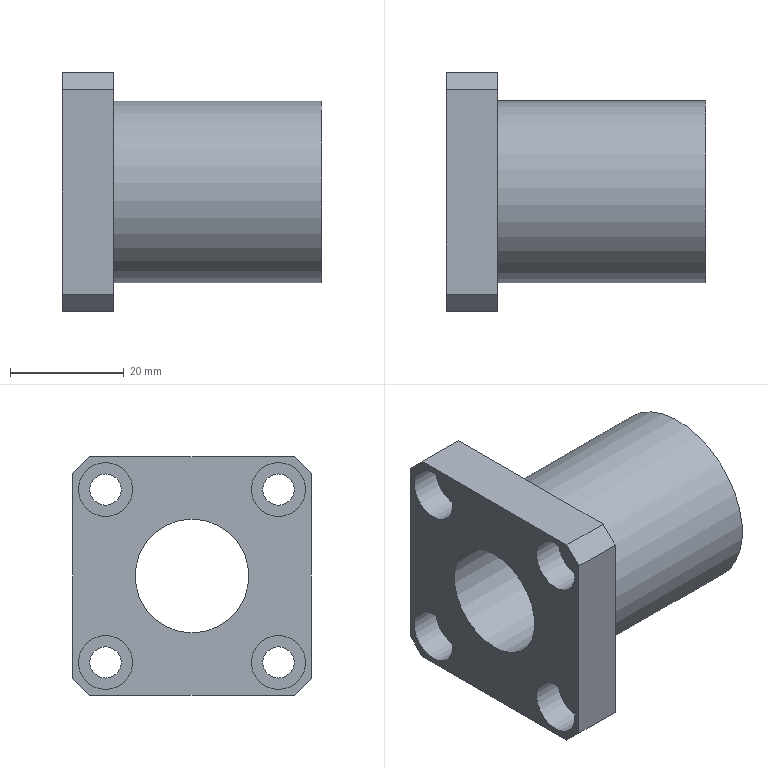Part | STEP file | Tube feed_id370_x_t | 1 solid | 25 faces | box 45.6 x 42 x 42 mm | volume 28951 mm3 | plane 15 | cylinder 10 | commonest cylinder face diameters 5.5 x4 9.5 x4 20 x1 32 x1